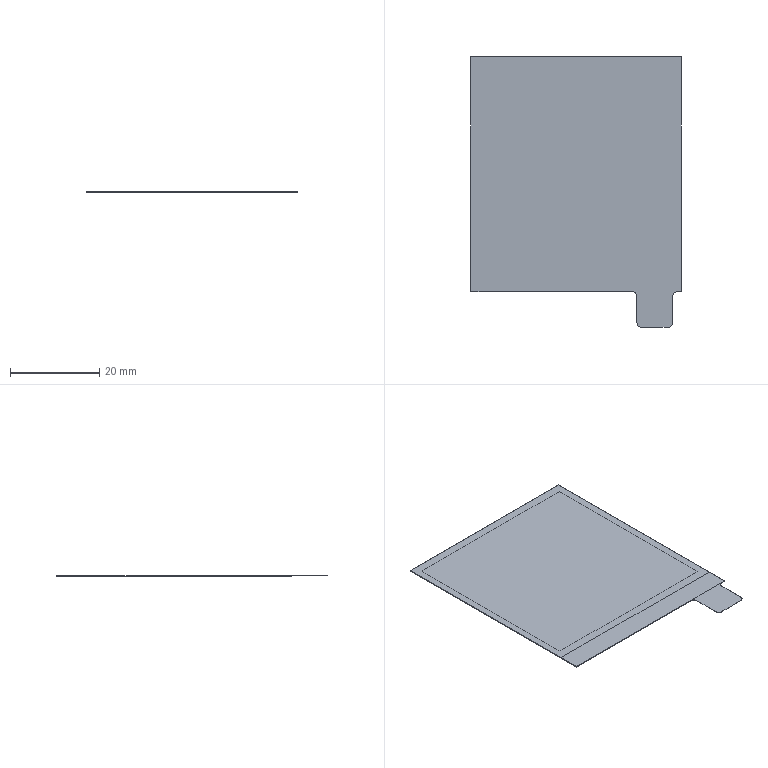Part | NX | features DATUM_CSYS 6, EXTRUDE 6, SKETCH 5 | 4 solids | 40 faces | box 47.2 x 60.8 x 0.18 mm | volume 184.569 mm3 | plane 36 | cylinder 4 | commonest cylinder face diameters 2 x4
STEP:
#1=CARTESIAN_POINT('',(0.,52.8,0.));
#2=VERTEX_POINT('',#1);
#3=CARTESIAN_POINT('',(0.,0.,0.));
#4=VERTEX_POINT('',#3);
#5=CARTESIAN_POINT('',(0.,52.8,0.));
#6=DIRECTION('',(0.,-1.,0.));
#7=VECTOR('',#6,1000.);
#8=LINE('',#5,#7);
#9=EDGE_CURVE('',#2,#4,#8,.T.);
#10=ORIENTED_EDGE('',*,*,#9,.F.);
#11=CARTESIAN_POINT('',(0.,52.8,-0.04));
#12=VERTEX_POINT('',#11);
#13=CARTESIAN_POINT('',(0.,52.8,-0.04));
#14=DIRECTION('',(0.,0.,1.));
#15=VECTOR('',#14,1000.);
#16=LINE('',#13,#15);
#17=EDGE_CURVE('',#12,#2,#16,.T.);
#18=ORIENTED_EDGE('',*,*,#17,.F.);
#19=CARTESIAN_POINT('',(0.,0.,-0.04));
#20=VERTEX_POINT('',#19);
#21=CARTESIAN_POINT('',(0.,52.8,-0.04));
#22=DIRECTION('',(0.,-1.,0.));
#23=VECTOR('',#22,1000.);
#24=LINE('',#21,#23);
#25=EDGE_CURVE('',#12,#20,#24,.T.);
#26=ORIENTED_EDGE('',*,*,#25,.T.);
#27=CARTESIAN_POINT('',(0.,0.,-0.04));
#28=DIRECTION('',(0.,0.,1.));
#29=VECTOR('',#28,1000.);
#30=LINE('',#27,#29);
#31=EDGE_CURVE('',#20,#4,#30,.T.);
#32=ORIENTED_EDGE('',*,*,#31,.T.);
#33=EDGE_LOOP('',(#10,#18,#26,#32));
#34=FACE_BOUND('',#33,.T.);
#35=CARTESIAN_POINT('',(0.,52.8,-0.04));
#36=DIRECTION('',(-1.,0.,0.));
#37=DIRECTION('',(0.,-1.,0.));
#38=AXIS2_PLACEMENT_3D('',#35,#36,#37);
#39=PLANE('',#38);
#40=ADVANCED_FACE('',(#34),#39,.T.);
#41=CARTESIAN_POINT('',(47.2,0.,0.));
#42=VERTEX_POINT('',#41);
#43=CARTESIAN_POINT('',(0.,0.,0.));
#44=DIRECTION('',(1.,0.,0.));
#45=VECTOR('',#44,1000.);
#46=LINE('',#43,#45);
#47=EDGE_CURVE('',#4,#42,#46,.T.);
#48=ORIENTED_EDGE('',*,*,#47,.F.);
#49=ORIENTED_EDGE('',*,*,#31,.F.);
#50=CARTESIAN_POINT('',(47.2,0.,-0.04));
#51=VERTEX_POINT('',#50);
#52=CARTESIAN_POINT('',(0.,0.,-0.04));
#53=DIRECTION('',(1.,0.,0.));
#54=VECTOR('',#53,1000.);
#55=LINE('',#52,#54);
#56=EDGE_CURVE('',#20,#51,#55,.T.);
#57=ORIENTED_EDGE('',*,*,#56,.T.);
#58=CARTESIAN_POINT('',(47.2,0.,-0.04));
#59=DIRECTION('',(0.,0.,1.));
#60=VECTOR('',#59,1000.);
#61=LINE('',#58,#60);
#62=EDGE_CURVE('',#51,#42,#61,.T.);
#63=ORIENTED_EDGE('',*,*,#62,.T.);
#64=EDGE_LOOP('',(#48,#49,#57,#63));
#65=FACE_BOUND('',#64,.T.);
#66=CARTESIAN_POINT('',(0.,0.,-0.04));
#67=DIRECTION('',(0.,-1.,0.));
#68=DIRECTION('',(0.,0.,-1.));
#69=AXIS2_PLACEMENT_3D('',#66,#67,#68);
#70=PLANE('',#69);
#71=ADVANCED_FACE('',(#65),#70,.T.);
#72=CARTESIAN_POINT('',(47.2,52.8,0.));
#73=VERTEX_POINT('',#72);
#74=CARTESIAN_POINT('',(47.2,0.,0.));
#75=DIRECTION('',(0.,1.,0.));
#76=VECTOR('',#75,1000.);
#77=LINE('',#74,#76);
#78=EDGE_CURVE('',#42,#73,#77,.T.);
#79=ORIENTED_EDGE('',*,*,#78,.F.);
#80=ORIENTED_EDGE('',*,*,#62,.F.);
#81=CARTESIAN_POINT('',(47.2,52.8,-0.04));
#82=VERTEX_POINT('',#81);
#83=CARTESIAN_POINT('',(47.2,0.,-0.04));
#84=DIRECTION('',(0.,1.,0.));
#85=VECTOR('',#84,1000.);
#86=LINE('',#83,#85);
#87=EDGE_CURVE('',#51,#82,#86,.T.);
#88=ORIENTED_EDGE('',*,*,#87,.T.);
#89=CARTESIAN_POINT('',(47.2,52.8,-0.04));
#90=DIRECTION('',(0.,0.,1.));
#91=VECTOR('',#90,1000.);
#92=LINE('',#89,#91);
#93=EDGE_CURVE('',#82,#73,#92,.T.);
#94=ORIENTED_EDGE('',*,*,#93,.T.);
#95=EDGE_LOOP('',(#79,#80,#88,#94));
#96=FACE_BOUND('',#95,.T.);
#97=CARTESIAN_POINT('',(47.2,0.,-0.04));
#98=DIRECTION('',(1.,0.,0.));
#99=DIRECTION('',(0.,0.,-1.));
#100=AXIS2_PLACEMENT_3D('',#97,#98,#99);
#101=PLANE('',#100);
#102=ADVANCED_FACE('',(#96),#101,.T.);
#103=CARTESIAN_POINT('',(47.2,52.8,0.));
#104=DIRECTION('',(-1.,0.,0.));
#105=VECTOR('',#104,1000.);
#106=LINE('',#103,#105);
#107=EDGE_CURVE('',#73,#2,#106,.T.);
#108=ORIENTED_EDGE('',*,*,#107,.F.);
#109=ORIENTED_EDGE('',*,*,#93,.F.);
#110=CARTESIAN_POINT('',(47.2,52.8,-0.04));
#111=DIRECTION('',(-1.,0.,0.));
#112=VECTOR('',#111,1000.);
#113=LINE('',#110,#112);
#114=EDGE_CURVE('',#82,#12,#113,.T.);
#115=ORIENTED_EDGE('',*,*,#114,.T.);
#116=ORIENTED_EDGE('',*,*,#17,.T.);
#117=EDGE_LOOP('',(#108,#109,#115,#116));
#118=FACE_BOUND('',#117,.T.);
#119=CARTESIAN_POINT('',(47.2,52.8,-0.04));
#120=DIRECTION('',(0.,1.,0.));
#121=DIRECTION('',(-1.,0.,0.));
#122=AXIS2_PLACEMENT_3D('',#119,#120,#121);
#123=PLANE('',#122);
#124=ADVANCED_FACE('',(#118),#123,.T.);
#125=CARTESIAN_POINT('',(45.5,50.9,-0.04));
#126=VERTEX_POINT('',#125);
#127=CARTESIAN_POINT('',(1.7,50.9,-0.04));
#128=VERTEX_POINT('',#127);
#129=CARTESIAN_POINT('',(0.,50.9,-0.04));
#130=DIRECTION('',(-1.,0.,0.));
#131=VECTOR('',#130,1000.);
#132=LINE('',#129,#131);
#133=EDGE_CURVE('',#126,#128,#132,.T.);
#134=ORIENTED_EDGE('',*,*,#133,.T.);
#135=CARTESIAN_POINT('',(1.7,6.9,-0.04));
#136=VERTEX_POINT('',#135);
#137=CARTESIAN_POINT('',(1.7,0.,-0.04));
#138=DIRECTION('',(0.,-1.,0.));
#139=VECTOR('',#138,1000.);
#140=LINE('',#137,#139);
#141=EDGE_CURVE('',#128,#136,#140,.T.);
#142=ORIENTED_EDGE('',*,*,#141,.T.);
#143=CARTESIAN_POINT('',(45.5,6.9,-0.04));
#144=VERTEX_POINT('',#143);
#145=CARTESIAN_POINT('',(0.,6.9,-0.04));
#146=DIRECTION('',(1.,0.,0.));
#147=VECTOR('',#146,1000.);
#148=LINE('',#145,#147);
#149=EDGE_CURVE('',#136,#144,#148,.T.);
#150=ORIENTED_EDGE('',*,*,#149,.T.);
#151=CARTESIAN_POINT('',(45.5,0.,-0.04));
#152=DIRECTION('',(0.,1.,0.));
#153=VECTOR('',#152,1000.);
#154=LINE('',#151,#153);
#155=EDGE_CURVE('',#144,#126,#154,.T.);
#156=ORIENTED_EDGE('',*,*,#155,.T.);
#157=EDGE_LOOP('',(#134,#142,#150,#156));
#158=FACE_BOUND('',#157,.T.);
#159=ORIENTED_EDGE('',*,*,#25,.F.);
#160=ORIENTED_EDGE('',*,*,#114,.F.);
#161=ORIENTED_EDGE('',*,*,#87,.F.);
#162=ORIENTED_EDGE('',*,*,#56,.F.);
#163=EDGE_LOOP('',(#159,#160,#161,#162));
#164=FACE_BOUND('',#163,.T.);
#165=CARTESIAN_POINT('',(0.,0.,-0.04));
#166=DIRECTION('',(0.,0.,1.));
#167=DIRECTION('',(1.,0.,0.));
#168=AXIS2_PLACEMENT_3D('',#165,#166,#167);
#169=PLANE('',#168);
#170=ADVANCED_FACE('',(#158,#164),#169,.F.);
#171=CARTESIAN_POINT('',(1.7,50.9,0.));
#172=VERTEX_POINT('',#171);
#173=CARTESIAN_POINT('',(1.7,6.9,0.));
#174=VERTEX_POINT('',#173);
#175=CARTESIAN_POINT('',(1.7,0.,0.));
#176=DIRECTION('',(0.,-1.,0.));
#177=VECTOR('',#176,1000.);
#178=LINE('',#175,#177);
#179=EDGE_CURVE('',#172,#174,#178,.T.);
#180=ORIENTED_EDGE('',*,*,#179,.F.);
#181=CARTESIAN_POINT('',(45.5,50.9,0.));
#182=VERTEX_POINT('',#181);
#183=CARTESIAN_POINT('',(0.,50.9,0.));
#184=DIRECTION('',(-1.,0.,0.));
#185=VECTOR('',#184,1000.);
#186=LINE('',#183,#185);
#187=EDGE_CURVE('',#182,#172,#186,.T.);
#188=ORIENTED_EDGE('',*,*,#187,.F.);
#189=CARTESIAN_POINT('',(45.5,6.9,0.));
#190=VERTEX_POINT('',#189);
#191=CARTESIAN_POINT('',(45.5,0.,0.));
#192=DIRECTION('',(0.,1.,0.));
#193=VECTOR('',#192,1000.);
#194=LINE('',#191,#193);
#195=EDGE_CURVE('',#190,#182,#194,.T.);
#196=ORIENTED_EDGE('',*,*,#195,.F.);
#197=CARTESIAN_POINT('',(0.,6.9,0.));
#198=DIRECTION('',(1.,0.,0.));
#199=VECTOR('',#198,1000.);
#200=LINE('',#197,#199);
#201=EDGE_CURVE('',#174,#190,#200,.T.);
#202=ORIENTED_EDGE('',*,*,#201,.F.);
#203=EDGE_LOOP('',(#180,#188,#196,#202));
#204=FACE_BOUND('',#203,.T.);
#205=ORIENTED_EDGE('',*,*,#9,.T.);
#206=ORIENTED_EDGE('',*,*,#47,.T.);
#207=ORIENTED_EDGE('',*,*,#78,.T.);
#208=ORIENTED_EDGE('',*,*,#107,.T.);
#209=EDGE_LOOP('',(#205,#206,#207,#208));
#210=FACE_BOUND('',#209,.T.);
#211=CARTESIAN_POINT('',(0.,0.,0.));
#212=DIRECTION('',(0.,0.,1.));
#213=DIRECTION('',(1.,0.,0.));
#214=AXIS2_PLACEMENT_3D('',#211,#212,#213);
#215=PLANE('',#214);
#216=ADVANCED_FACE('',(#204,#210),#215,.T.);
#217=CARTESIAN_POINT('',(1.7,50.9,1.05));
#218=DIRECTION('',(0.,0.,-1.));
#219=VECTOR('',#218,1000.);
#220=LINE('',#217,#219);
#221=EDGE_CURVE('',#128,#172,#220,.F.);
#222=ORIENTED_EDGE('',*,*,#221,.T.);
#223=ORIENTED_EDGE('',*,*,#179,.T.);
#224=CARTESIAN_POINT('',(1.7,6.9,1.05));
#225=DIRECTION('',(0.,0.,-1.));
#226=VECTOR('',#225,1000.);
#227=LINE('',#224,#226);
#228=EDGE_CURVE('',#136,#174,#227,.F.);
#229=ORIENTED_EDGE('',*,*,#228,.F.);
#230=ORIENTED_EDGE('',*,*,#141,.F.);
#231=EDGE_LOOP('',(#222,#223,#229,#230));
#232=FACE_BOUND('',#231,.T.);
#233=CARTESIAN_POINT('',(1.7,6.9,1.05));
#234=DIRECTION('',(-1.,0.,0.));
#235=DIRECTION('',(0.,-1.,0.));
#236=AXIS2_PLACEMENT_3D('',#233,#234,#235);
#237=PLANE('',#236);
#238=ADVANCED_FACE('',(#232),#237,.F.);
#239=CARTESIAN_POINT('',(45.5,50.9,1.05));
#240=DIRECTION('',(0.,0.,-1.));
#241=VECTOR('',#240,1000.);
#242=LINE('',#239,#241);
#243=EDGE_CURVE('',#126,#182,#242,.F.);
#244=ORIENTED_EDGE('',*,*,#243,.T.);
#245=ORIENTED_EDGE('',*,*,#187,.T.);
#246=ORIENTED_EDGE('',*,*,#221,.F.);
#247=ORIENTED_EDGE('',*,*,#133,.F.);
#248=EDGE_LOOP('',(#244,#245,#246,#247));
#249=FACE_BOUND('',#248,.T.);
#250=CARTESIAN_POINT('',(1.7,50.9,1.05));
#251=DIRECTION('',(0.,1.,0.));
#252=DIRECTION('',(-1.,0.,0.));
#253=AXIS2_PLACEMENT_3D('',#250,#251,#252);
#254=PLANE('',#253);
#255=ADVANCED_FACE('',(#249),#254,.F.);
#256=CARTESIAN_POINT('',(45.5,6.9,1.05));
#257=DIRECTION('',(0.,0.,-1.));
#258=VECTOR('',#257,1000.);
#259=LINE('',#256,#258);
#260=EDGE_CURVE('',#144,#190,#259,.F.);
#261=ORIENTED_EDGE('',*,*,#260,.T.);
#262=ORIENTED_EDGE('',*,*,#195,.T.);
#263=ORIENTED_EDGE('',*,*,#243,.F.);
#264=ORIENTED_EDGE('',*,*,#155,.F.);
#265=EDGE_LOOP('',(#261,#262,#263,#264));
#266=FACE_BOUND('',#265,.T.);
#267=CARTESIAN_POINT('',(45.5,50.9,1.05));
#268=DIRECTION('',(1.,0.,0.));
#269=DIRECTION('',(0.,1.,0.));
#270=AXIS2_PLACEMENT_3D('',#267,#268,#269);
#271=PLANE('',#270);
#272=ADVANCED_FACE('',(#266),#271,.F.);
#273=ORIENTED_EDGE('',*,*,#228,.T.);
#274=ORIENTED_EDGE('',*,*,#201,.T.);
#275=ORIENTED_EDGE('',*,*,#260,.F.);
#276=ORIENTED_EDGE('',*,*,#149,.F.);
#277=EDGE_LOOP('',(#273,#274,#275,#276));
#278=FACE_BOUND('',#277,.T.);
#279=CARTESIAN_POINT('',(45.5,6.9,1.05));
#280=DIRECTION('',(0.,-1.,0.));
#281=DIRECTION('',(1.,0.,0.));
#282=AXIS2_PLACEMENT_3D('',#279,#280,#281);
#283=PLANE('',#282);
#284=ADVANCED_FACE('',(#278),#283,.F.);
#285=CLOSED_SHELL('',(#40,#71,#102,#124,#170,#216,#238,#255,#272,#284));
#286=MANIFOLD_SOLID_BREP('',#285);
#287=CARTESIAN_POINT('',(0.,0.,-0.08));
#288=VERTEX_POINT('',#287);
#289=CARTESIAN_POINT('',(0.,52.8,-0.08));
#290=VERTEX_POINT('',#289);
#291=CARTESIAN_POINT('',(0.,0.,-0.08));
#292=DIRECTION('',(0.,1.,0.));
#293=VECTOR('',#292,1000.);
#294=LINE('',#291,#293);
#295=EDGE_CURVE('',#288,#290,#294,.T.);
#296=ORIENTED_EDGE('',*,*,#295,.T.);
#297=CARTESIAN_POINT('',(47.2,52.8,-0.08));
#298=VERTEX_POINT('',#297);
#299=CARTESIAN_POINT('',(0.,52.8,-0.08));
#300=DIRECTION('',(1.,0.,0.));
#301=VECTOR('',#300,1000.);
#302=LINE('',#299,#301);
#303=EDGE_CURVE('',#290,#298,#302,.T.);
#304=ORIENTED_EDGE('',*,*,#303,.T.);
#305=CARTESIAN_POINT('',(47.2,0.,-0.08));
#306=VERTEX_POINT('',#305);
#307=CARTESIAN_POINT('',(47.2,52.8,-0.08));
#308=DIRECTION('',(0.,-1.,0.));
#309=VECTOR('',#308,1000.);
#310=LINE('',#307,#309);
#311=EDGE_CURVE('',#298,#306,#310,.T.);
#312=ORIENTED_EDGE('',*,*,#311,.T.);
#313=CARTESIAN_POINT('',(47.2,0.,-0.08));
#314=DIRECTION('',(-1.,0.,0.));
#315=VECTOR('',#314,1000.);
#316=LINE('',#313,#315);
#317=EDGE_CURVE('',#306,#288,#316,.T.);
#318=ORIENTED_EDGE('',*,*,#317,.T.);
#319=EDGE_LOOP('',(#296,#304,#312,#318));
#320=FACE_BOUND('',#319,.T.);
#321=CARTESIAN_POINT('',(45.5,50.9,-0.08));
#322=VERTEX_POINT('',#321);
#323=CARTESIAN_POINT('',(1.7,50.9,-0.08));
#324=VERTEX_POINT('',#323);
#325=CARTESIAN_POINT('',(0.,50.9,-0.08));
#326=DIRECTION('',(-1.,0.,0.));
#327=VECTOR('',#326,1000.);
#328=LINE('',#325,#327);
#329=EDGE_CURVE('',#322,#324,#328,.T.);
#330=ORIENTED_EDGE('',*,*,#329,.T.);
#331=CARTESIAN_POINT('',(1.7,6.9,-0.08));
#332=VERTEX_POINT('',#331);
#333=CARTESIAN_POINT('',(1.7,0.,-0.08));
#334=DIRECTION('',(0.,-1.,0.));
#335=VECTOR('',#334,1000.);
#336=LINE('',#333,#335);
#337=EDGE_CURVE('',#324,#332,#336,.T.);
#338=ORIENTED_EDGE('',*,*,#337,.T.);
#339=CARTESIAN_POINT('',(45.5,6.9,-0.08));
#340=VERTEX_POINT('',#339);
#341=CARTESIAN_POINT('',(0.,6.9,-0.08));
#342=DIRECTION('',(1.,0.,0.));
#343=VECTOR('',#342,1000.);
#344=LINE('',#341,#343);
#345=EDGE_CURVE('',#332,#340,#344,.T.);
#346=ORIENTED_EDGE('',*,*,#345,.T.);
#347=CARTESIAN_POINT('',(45.5,0.,-0.08));
#348=DIRECTION('',(0.,1.,0.));
#349=VECTOR('',#348,1000.);
#350=LINE('',#347,#349);
#351=EDGE_CURVE('',#340,#322,#350,.T.);
#352=ORIENTED_EDGE('',*,*,#351,.T.);
#353=EDGE_LOOP('',(#330,#338,#346,#352));
#354=FACE_BOUND('',#353,.T.);
#355=CARTESIAN_POINT('',(0.,0.,-0.08));
#356=DIRECTION('',(0.,0.,-1.));
#357=DIRECTION('',(-1.,0.,0.));
#358=AXIS2_PLACEMENT_3D('',#355,#356,#357);
#359=PLANE('',#358);
#360=ADVANCED_FACE('',(#320,#354),#359,.T.);
#361=CARTESIAN_POINT('',(0.,0.,-0.04));
#362=VERTEX_POINT('',#361);
#363=CARTESIAN_POINT('',(0.,52.8,-0.04));
#364=VERTEX_POINT('',#363);
#365=CARTESIAN_POINT('',(0.,0.,-0.04));
#366=DIRECTION('',(0.,1.,0.));
#367=VECTOR('',#366,1000.);
#368=LINE('',#365,#367);
#369=EDGE_CURVE('',#362,#364,#368,.T.);
#370=ORIENTED_EDGE('',*,*,#369,.F.);
#371=CARTESIAN_POINT('',(47.2,0.,-0.04));
#372=VERTEX_POINT('',#371);
#373=CARTESIAN_POINT('',(47.2,0.,-0.04));
#374=DIRECTION('',(-1.,0.,0.));
#375=VECTOR('',#374,1000.);
#376=LINE('',#373,#375);
#377=EDGE_CURVE('',#372,#362,#376,.T.);
#378=ORIENTED_EDGE('',*,*,#377,.F.);
#379=CARTESIAN_POINT('',(47.2,52.8,-0.04));
#380=VERTEX_POINT('',#379);
#381=CARTESIAN_POINT('',(47.2,52.8,-0.04));
#382=DIRECTION('',(0.,-1.,0.));
#383=VECTOR('',#382,1000.);
#384=LINE('',#381,#383);
#385=EDGE_CURVE('',#380,#372,#384,.T.);
#386=ORIENTED_EDGE('',*,*,#385,.F.);
#387=CARTESIAN_POINT('',(0.,52.8,-0.04));
#388=DIRECTION('',(1.,0.,0.));
#389=VECTOR('',#388,1000.);
#390=LINE('',#387,#389);
#391=EDGE_CURVE('',#364,#380,#390,.T.);
#392=ORIENTED_EDGE('',*,*,#391,.F.);
#393=EDGE_LOOP('',(#370,#378,#386,#392));
#394=FACE_BOUND('',#393,.T.);
#395=CARTESIAN_POINT('',(1.7,50.9,-0.04));
#396=VERTEX_POINT('',#395);
#397=CARTESIAN_POINT('',(1.7,6.9,-0.04));
#398=VERTEX_POINT('',#397);
#399=CARTESIAN_POINT('',(1.7,0.,-0.04));
#400=DIRECTION('',(0.,-1.,0.));
#401=VECTOR('',#400,1000.);
#402=LINE('',#399,#401);
#403=EDGE_CURVE('',#396,#398,#402,.T.);
#404=ORIENTED_EDGE('',*,*,#403,.F.);
#405=CARTESIAN_POINT('',(45.5,50.9,-0.04));
#406=VERTEX_POINT('',#405);
#407=CARTESIAN_POINT('',(0.,50.9,-0.04));
#408=DIRECTION('',(-1.,0.,0.));
#409=VECTOR('',#408,1000.);
#410=LINE('',#407,#409);
#411=EDGE_CURVE('',#406,#396,#410,.T.);
#412=ORIENTED_EDGE('',*,*,#411,.F.);
#413=CARTESIAN_POINT('',(45.5,6.9,-0.04));
#414=VERTEX_POINT('',#413);
#415=CARTESIAN_POINT('',(45.5,0.,-0.04));
#416=DIRECTION('',(0.,1.,0.));
#417=VECTOR('',#416,1000.);
#418=LINE('',#415,#417);
#419=EDGE_CURVE('',#414,#406,#418,.T.);
#420=ORIENTED_EDGE('',*,*,#419,.F.);
#421=CARTESIAN_POINT('',(0.,6.9,-0.04));
#422=DIRECTION('',(1.,0.,0.));
#423=VECTOR('',#422,1000.);
#424=LINE('',#421,#423);
#425=EDGE_CURVE('',#398,#414,#424,.T.);
#426=ORIENTED_EDGE('',*,*,#425,.F.);
#427=EDGE_LOOP('',(#404,#412,#420,#426));
#428=FACE_BOUND('',#427,.T.);
#429=CARTESIAN_POINT('',(0.,0.,-0.04));
#430=DIRECTION('',(0.,0.,-1.));
#431=DIRECTION('',(-1.,0.,0.));
#432=AXIS2_PLACEMENT_3D('',#429,#430,#431);
#433=PLANE('',#432);
#434=ADVANCED_FACE('',(#394,#428),#433,.F.);
#435=ORIENTED_EDGE('',*,*,#369,.T.);
#436=CARTESIAN_POINT('',(0.,52.8,-0.08));
#437=DIRECTION('',(0.,0.,1.));
#438=VECTOR('',#437,1000.);
#439=LINE('',#436,#438);
#440=EDGE_CURVE('',#290,#364,#439,.T.);
#441=ORIENTED_EDGE('',*,*,#440,.F.);
#442=ORIENTED_EDGE('',*,*,#295,.F.);
#443=CARTESIAN_POINT('',(0.,0.,-0.08));
#444=DIRECTION('',(0.,0.,1.));
#445=VECTOR('',#444,1000.);
#446=LINE('',#443,#445);
#447=EDGE_CURVE('',#288,#362,#446,.T.);
#448=ORIENTED_EDGE('',*,*,#447,.T.);
#449=EDGE_LOOP('',(#435,#441,#442,#448));
#450=FACE_BOUND('',#449,.T.);
#451=CARTESIAN_POINT('',(0.,0.,-0.08));
#452=DIRECTION('',(1.,0.,0.));
#453=DIRECTION('',(0.,0.,-1.));
#454=AXIS2_PLACEMENT_3D('',#451,#452,#453);
#455=PLANE('',#454);
#456=ADVANCED_FACE('',(#450),#455,.F.);
#457=ORIENTED_EDGE('',*,*,#391,.T.);
#458=CARTESIAN_POINT('',(47.2,52.8,-0.08));
#459=DIRECTION('',(0.,0.,1.));
#460=VECTOR('',#459,1000.);
#461=LINE('',#458,#460);
#462=EDGE_CURVE('',#298,#380,#461,.T.);
#463=ORIENTED_EDGE('',*,*,#462,.F.);
#464=ORIENTED_EDGE('',*,*,#303,.F.);
#465=ORIENTED_EDGE('',*,*,#440,.T.);
#466=EDGE_LOOP('',(#457,#463,#464,#465));
#467=FACE_BOUND('',#466,.T.);
#468=CARTESIAN_POINT('',(0.,52.8,-0.08));
#469=DIRECTION('',(0.,-1.,0.));
#470=DIRECTION('',(0.,0.,-1.));
#471=AXIS2_PLACEMENT_3D('',#468,#469,#470);
#472=PLANE('',#471);
#473=ADVANCED_FACE('',(#467),#472,.F.);
#474=ORIENTED_EDGE('',*,*,#385,.T.);
#475=CARTESIAN_POINT('',(47.2,0.,-0.08));
#476=DIRECTION('',(0.,0.,1.));
#477=VECTOR('',#476,1000.);
#478=LINE('',#475,#477);
#479=EDGE_CURVE('',#306,#372,#478,.T.);
#480=ORIENTED_EDGE('',*,*,#479,.F.);
#481=ORIENTED_EDGE('',*,*,#311,.F.);
#482=ORIENTED_EDGE('',*,*,#462,.T.);
#483=EDGE_LOOP('',(#474,#480,#481,#482));
#484=FACE_BOUND('',#483,.T.);
#485=CARTESIAN_POINT('',(47.2,52.8,-0.08));
#486=DIRECTION('',(-1.,0.,0.));
#487=DIRECTION('',(0.,0.,1.));
#488=AXIS2_PLACEMENT_3D('',#485,#486,#487);
#489=PLANE('',#488);
#490=ADVANCED_FACE('',(#484),#489,.F.);
#491=ORIENTED_EDGE('',*,*,#377,.T.);
#492=ORIENTED_EDGE('',*,*,#447,.F.);
#493=ORIENTED_EDGE('',*,*,#317,.F.);
#494=ORIENTED_EDGE('',*,*,#479,.T.);
#495=EDGE_LOOP('',(#491,#492,#493,#494));
#496=FACE_BOUND('',#495,.T.);
#497=CARTESIAN_POINT('',(47.2,0.,-0.08));
#498=DIRECTION('',(0.,1.,0.));
#499=DIRECTION('',(0.,0.,1.));
#500=AXIS2_PLACEMENT_3D('',#497,#498,#499);
#501=PLANE('',#500);
#502=ADVANCED_FACE('',(#496),#501,.F.);
#503=CARTESIAN_POINT('',(1.7,50.9,1.05));
#504=DIRECTION('',(0.,0.,-1.));
#505=VECTOR('',#504,1000.);
#506=LINE('',#503,#505);
#507=EDGE_CURVE('',#324,#396,#506,.F.);
#508=ORIENTED_EDGE('',*,*,#507,.T.);
#509=ORIENTED_EDGE('',*,*,#403,.T.);
#510=CARTESIAN_POINT('',(1.7,6.9,1.05));
#511=DIRECTION('',(0.,0.,-1.));
#512=VECTOR('',#511,1000.);
#513=LINE('',#510,#512);
#514=EDGE_CURVE('',#332,#398,#513,.F.);
#515=ORIENTED_EDGE('',*,*,#514,.F.);
#516=ORIENTED_EDGE('',*,*,#337,.F.);
#517=EDGE_LOOP('',(#508,#509,#515,#516));
#518=FACE_BOUND('',#517,.T.);
#519=CARTESIAN_POINT('',(1.7,50.9,1.05));
#520=DIRECTION('',(1.,0.,0.));
#521=DIRECTION('',(0.,1.,0.));
#522=AXIS2_PLACEMENT_3D('',#519,#520,#521);
#523=PLANE('',#522);
#524=ADVANCED_FACE('',(#518),#523,.T.);
#525=ORIENTED_EDGE('',*,*,#514,.T.);
#526=ORIENTED_EDGE('',*,*,#425,.T.);
#527=CARTESIAN_POINT('',(45.5,6.9,1.05));
#528=DIRECTION('',(0.,0.,-1.));
#529=VECTOR('',#528,1000.);
#530=LINE('',#527,#529);
#531=EDGE_CURVE('',#340,#414,#530,.F.);
#532=ORIENTED_EDGE('',*,*,#531,.F.);
#533=ORIENTED_EDGE('',*,*,#345,.F.);
#534=EDGE_LOOP('',(#525,#526,#532,#533));
#535=FACE_BOUND('',#534,.T.);
#536=CARTESIAN_POINT('',(1.7,6.9,1.05));
#537=DIRECTION('',(0.,1.,0.));
#538=DIRECTION('',(-1.,0.,0.));
#539=AXIS2_PLACEMENT_3D('',#536,#537,#538);
#540=PLANE('',#539);
#541=ADVANCED_FACE('',(#535),#540,.T.);
#542=ORIENTED_EDGE('',*,*,#531,.T.);
#543=ORIENTED_EDGE('',*,*,#419,.T.);
#544=CARTESIAN_POINT('',(45.5,50.9,1.05));
#545=DIRECTION('',(0.,0.,-1.));
#546=VECTOR('',#545,1000.);
#547=LINE('',#544,#546);
#548=EDGE_CURVE('',#322,#406,#547,.F.);
#549=ORIENTED_EDGE('',*,*,#548,.F.);
#550=ORIENTED_EDGE('',*,*,#351,.F.);
#551=EDGE_LOOP('',(#542,#543,#549,#550));
#552=FACE_BOUND('',#551,.T.);
#553=CARTESIAN_POINT('',(45.5,6.9,1.05));
#554=DIRECTION('',(-1.,0.,0.));
#555=DIRECTION('',(0.,-1.,0.));
#556=AXIS2_PLACEMENT_3D('',#553,#554,#555);
#557=PLANE('',#556);
#558=ADVANCED_FACE('',(#552),#557,.T.);
#559=ORIENTED_EDGE('',*,*,#548,.T.);
#560=ORIENTED_EDGE('',*,*,#411,.T.);
#561=ORIENTED_EDGE('',*,*,#507,.F.);
#562=ORIENTED_EDGE('',*,*,#329,.F.);
#563=EDGE_LOOP('',(#559,#560,#561,#562));
#564=FACE_BOUND('',#563,.T.);
#565=CARTESIAN_POINT('',(45.5,50.9,1.05));
#566=DIRECTION('',(0.,-1.,0.));
#567=DIRECTION('',(1.,0.,0.));
#568=AXIS2_PLACEMENT_3D('',#565,#566,#567);
#569=PLANE('',#568);
#570=ADVANCED_FACE('',(#564),#569,.T.);
#571=CLOSED_SHELL('',(#360,#434,#456,#473,#490,#502,#524,#541,#558,#570));
#572=MANIFOLD_SOLID_BREP('',#571);
#573=CARTESIAN_POINT('',(0.,52.8,0.05));
#574=VERTEX_POINT('',#573);
#575=CARTESIAN_POINT('',(0.,0.,0.05));
#576=VERTEX_POINT('',#575);
#577=CARTESIAN_POINT('',(0.,52.8,0.05));
#578=DIRECTION('',(0.,-1.,0.));
#579=VECTOR('',#578,1000.);
#580=LINE('',#577,#579);
#581=EDGE_CURVE('',#574,#576,#580,.T.);
#582=ORIENTED_EDGE('',*,*,#581,.T.);
#583=CARTESIAN_POINT('',(0.,0.,0.1));
#584=VERTEX_POINT('',#583);
#585=CARTESIAN_POINT('',(0.,0.,0.1));
#586=DIRECTION('',(0.,0.,-1.));
#587=VECTOR('',#586,1000.);
#588=LINE('',#585,#587);
#589=EDGE_CURVE('',#584,#576,#588,.T.);
#590=ORIENTED_EDGE('',*,*,#589,.F.);
#591=CARTESIAN_POINT('',(0.,52.8,0.1));
#592=VERTEX_POINT('',#591);
#593=CARTESIAN_POINT('',(0.,52.8,0.1));
#594=DIRECTION('',(0.,-1.,0.));
#595=VECTOR('',#594,1000.);
#596=LINE('',#593,#595);
#597=EDGE_CURVE('',#592,#584,#596,.T.);
#598=ORIENTED_EDGE('',*,*,#597,.F.);
#599=CARTESIAN_POINT('',(0.,52.8,0.1));
#600=DIRECTION('',(0.,0.,-1.));
#601=VECTOR('',#600,1000.);
#602=LINE('',#599,#601);
#603=EDGE_CURVE('',#592,#574,#602,.T.);
#604=ORIENTED_EDGE('',*,*,#603,.T.);
#605=EDGE_LOOP('',(#582,#590,#598,#604));
#606=FACE_BOUND('',#605,.T.);
#607=CARTESIAN_POINT('',(0.,52.8,0.1));
#608=DIRECTION('',(1.,0.,0.));
#609=DIRECTION('',(0.,0.,-1.));
#610=AXIS2_PLACEMENT_3D('',#607,#608,#609);
#611=PLANE('',#610);
#612=ADVANCED_FACE('',(#606),#611,.F.);
#613=CARTESIAN_POINT('',(36.3,0.,0.05));
#614=VERTEX_POINT('',#613);
#615=CARTESIAN_POINT('',(0.,0.,0.05));
#616=DIRECTION('',(1.,0.,0.));
#617=VECTOR('',#616,1000.);
#618=LINE('',#615,#617);
#619=EDGE_CURVE('',#576,#614,#618,.T.);
#620=ORIENTED_EDGE('',*,*,#619,.T.);
#621=CARTESIAN_POINT('',(36.3,0.,0.1));
#622=VERTEX_POINT('',#621);
#623=CARTESIAN_POINT('',(36.3,0.,0.1));
#624=DIRECTION('',(0.,0.,-1.));
#625=VECTOR('',#624,1000.);
#626=LINE('',#623,#625);
#627=EDGE_CURVE('',#622,#614,#626,.T.);
#628=ORIENTED_EDGE('',*,*,#627,.F.);
#629=CARTESIAN_POINT('',(0.,0.,0.1));
#630=DIRECTION('',(1.,0.,0.));
#631=VECTOR('',#630,1000.);
#632=LINE('',#629,#631);
#633=EDGE_CURVE('',#584,#622,#632,.T.);
#634=ORIENTED_EDGE('',*,*,#633,.F.);
#635=ORIENTED_EDGE('',*,*,#589,.T.);
#636=EDGE_LOOP('',(#620,#628,#634,#635));
#637=FACE_BOUND('',#636,.T.);
#638=CARTESIAN_POINT('',(0.,0.,0.1));
#639=DIRECTION('',(0.,1.,0.));
#640=DIRECTION('',(0.,0.,1.));
#641=AXIS2_PLACEMENT_3D('',#638,#639,#640);
#642=PLANE('',#641);
#643=ADVANCED_FACE('',(#637),#642,.F.);
#644=CARTESIAN_POINT('',(37.3,-1.,0.05));
#645=VERTEX_POINT('',#644);
#646=CARTESIAN_POINT('',(36.3,-1.,0.05));
#647=DIRECTION('',(0.,0.,-1.));
#648=DIRECTION('',(0.,1.,0.));
#649=AXIS2_PLACEMENT_3D('',#646,#647,#648);
#650=CIRCLE('',#649,1.);
#651=EDGE_CURVE('',#614,#645,#650,.T.);
#652=ORIENTED_EDGE('',*,*,#651,.T.);
#653=CARTESIAN_POINT('',(37.3,-1.,0.1));
#654=VERTEX_POINT('',#653);
#655=CARTESIAN_POINT('',(37.3,-1.,0.1));
#656=DIRECTION('',(0.,0.,-1.));
#657=VECTOR('',#656,1000.);
#658=LINE('',#655,#657);
#659=EDGE_CURVE('',#654,#645,#658,.T.);
#660=ORIENTED_EDGE('',*,*,#659,.F.);
#661=CARTESIAN_POINT('',(36.3,-1.,0.1));
#662=DIRECTION('',(0.,0.,-1.));
#663=DIRECTION('',(0.,1.,0.));
#664=AXIS2_PLACEMENT_3D('',#661,#662,#663);
#665=CIRCLE('',#664,1.);
#666=EDGE_CURVE('',#622,#654,#665,.T.);
#667=ORIENTED_EDGE('',*,*,#666,.F.);
#668=ORIENTED_EDGE('',*,*,#627,.T.);
#669=EDGE_LOOP('',(#652,#660,#667,#668));
#670=FACE_BOUND('',#669,.T.);
#671=CARTESIAN_POINT('',(36.3,-1.,0.1));
#672=DIRECTION('',(0.,0.,-1.));
#673=DIRECTION('',(-1.,0.,0.));
#674=AXIS2_PLACEMENT_3D('',#671,#672,#673);
#675=CYLINDRICAL_SURFACE('',#674,1.);
#676=ADVANCED_FACE('',(#670),#675,.F.);
#677=CARTESIAN_POINT('',(37.3,-7.,0.05));
#678=VERTEX_POINT('',#677);
#679=CARTESIAN_POINT('',(37.3,-1.,0.05));
#680=DIRECTION('',(0.,-1.,0.));
#681=VECTOR('',#680,1000.);
#682=LINE('',#679,#681);
#683=EDGE_CURVE('',#645,#678,#682,.T.);
#684=ORIENTED_EDGE('',*,*,#683,.T.);
#685=CARTESIAN_POINT('',(37.3,-7.,0.1));
#686=VERTEX_POINT('',#685);
#687=CARTESIAN_POINT('',(37.3,-7.,0.1));
#688=DIRECTION('',(0.,0.,-1.));
#689=VECTOR('',#688,1000.);
#690=LINE('',#687,#689);
#691=EDGE_CURVE('',#686,#678,#690,.T.);
#692=ORIENTED_EDGE('',*,*,#691,.F.);
#693=CARTESIAN_POINT('',(37.3,-1.,0.1));
#694=DIRECTION('',(0.,-1.,0.));
#695=VECTOR('',#694,1000.);
#696=LINE('',#693,#695);
#697=EDGE_CURVE('',#654,#686,#696,.T.);
#698=ORIENTED_EDGE('',*,*,#697,.F.);
#699=ORIENTED_EDGE('',*,*,#659,.T.);
#700=EDGE_LOOP('',(#684,#692,#698,#699));
#701=FACE_BOUND('',#700,.T.);
#702=CARTESIAN_POINT('',(37.3,-1.,0.1));
#703=DIRECTION('',(1.,0.,0.));
#704=DIRECTION('',(0.,1.,0.));
#705=AXIS2_PLACEMENT_3D('',#702,#703,#704);
#706=PLANE('',#705);
#707=ADVANCED_FACE('',(#701),#706,.F.);
#708=CARTESIAN_POINT('',(38.3,-8.,0.05));
#709=VERTEX_POINT('',#708);
#710=CARTESIAN_POINT('',(38.3,-7.,0.05));
#711=DIRECTION('',(0.,0.,1.));
#712=DIRECTION('',(0.,1.,0.));
#713=AXIS2_PLACEMENT_3D('',#710,#711,#712);
#714=CIRCLE('',#713,1.);
#715=EDGE_CURVE('',#678,#709,#714,.T.);
#716=ORIENTED_EDGE('',*,*,#715,.T.);
#717=CARTESIAN_POINT('',(38.3,-8.,0.1));
#718=VERTEX_POINT('',#717);
#719=CARTESIAN_POINT('',(38.3,-8.,0.1));
#720=DIRECTION('',(0.,0.,-1.));
#721=VECTOR('',#720,1000.);
#722=LINE('',#719,#721);
#723=EDGE_CURVE('',#718,#709,#722,.T.);
#724=ORIENTED_EDGE('',*,*,#723,.F.);
#725=CARTESIAN_POINT('',(38.3,-7.,0.1));
#726=DIRECTION('',(0.,0.,1.));
#727=DIRECTION('',(0.,1.,0.));
#728=AXIS2_PLACEMENT_3D('',#725,#726,#727);
#729=CIRCLE('',#728,1.);
#730=EDGE_CURVE('',#686,#718,#729,.T.);
#731=ORIENTED_EDGE('',*,*,#730,.F.);
#732=ORIENTED_EDGE('',*,*,#691,.T.);
#733=EDGE_LOOP('',(#716,#724,#731,#732));
#734=FACE_BOUND('',#733,.T.);
#735=CARTESIAN_POINT('',(38.3,-7.,0.1));
#736=DIRECTION('',(0.,0.,-1.));
#737=DIRECTION('',(-1.,0.,0.));
#738=AXIS2_PLACEMENT_3D('',#735,#736,#737);
#739=CYLINDRICAL_SURFACE('',#738,1.);
#740=ADVANCED_FACE('',(#734),#739,.T.);
#741=CARTESIAN_POINT('',(44.3,-8.,0.05));
#742=VERTEX_POINT('',#741);
#743=CARTESIAN_POINT('',(38.3,-8.,0.05));
#744=DIRECTION('',(1.,0.,0.));
#745=VECTOR('',#744,1000.);
#746=LINE('',#743,#745);
#747=EDGE_CURVE('',#709,#742,#746,.T.);
#748=ORIENTED_EDGE('',*,*,#747,.T.);
#749=CARTESIAN_POINT('',(44.3,-8.,0.1));
#750=VERTEX_POINT('',#749);
#751=CARTESIAN_POINT('',(44.3,-8.,0.1));
#752=DIRECTION('',(0.,0.,-1.));
#753=VECTOR('',#752,1000.);
#754=LINE('',#751,#753);
#755=EDGE_CURVE('',#750,#742,#754,.T.);
#756=ORIENTED_EDGE('',*,*,#755,.F.);
#757=CARTESIAN_POINT('',(38.3,-8.,0.1));
#758=DIRECTION('',(1.,0.,0.));
#759=VECTOR('',#758,1000.);
#760=LINE('',#757,#759);
#761=EDGE_CURVE('',#718,#750,#760,.T.);
#762=ORIENTED_EDGE('',*,*,#761,.F.);
#763=ORIENTED_EDGE('',*,*,#723,.T.);
#764=EDGE_LOOP('',(#748,#756,#762,#763));
#765=FACE_BOUND('',#764,.T.);
#766=CARTESIAN_POINT('',(38.3,-8.,0.1));
#767=DIRECTION('',(0.,1.,0.));
#768=DIRECTION('',(-1.,0.,0.));
#769=AXIS2_PLACEMENT_3D('',#766,#767,#768);
#770=PLANE('',#769);
#771=ADVANCED_FACE('',(#765),#770,.F.);
#772=CARTESIAN_POINT('',(45.3,-7.,0.05));
#773=VERTEX_POINT('',#772);
#774=CARTESIAN_POINT('',(44.3,-7.,0.05));
#775=DIRECTION('',(0.,0.,1.));
#776=DIRECTION('',(0.,1.,0.));
#777=AXIS2_PLACEMENT_3D('',#774,#775,#776);
#778=CIRCLE('',#777,1.);
#779=EDGE_CURVE('',#742,#773,#778,.T.);
#780=ORIENTED_EDGE('',*,*,#779,.T.);
#781=CARTESIAN_POINT('',(45.3,-7.,0.1));
#782=VERTEX_POINT('',#781);
#783=CARTESIAN_POINT('',(45.3,-7.,0.1));
#784=DIRECTION('',(0.,0.,-1.));
#785=VECTOR('',#784,1000.);
#786=LINE('',#783,#785);
#787=EDGE_CURVE('',#782,#773,#786,.T.);
#788=ORIENTED_EDGE('',*,*,#787,.F.);
#789=CARTESIAN_POINT('',(44.3,-7.,0.1));
#790=DIRECTION('',(0.,0.,1.));
#791=DIRECTION('',(0.,1.,0.));
#792=AXIS2_PLACEMENT_3D('',#789,#790,#791);
#793=CIRCLE('',#792,1.);
#794=EDGE_CURVE('',#750,#782,#793,.T.);
#795=ORIENTED_EDGE('',*,*,#794,.F.);
#796=ORIENTED_EDGE('',*,*,#755,.T.);
#797=EDGE_LOOP('',(#780,#788,#795,#796));
#798=FACE_BOUND('',#797,.T.);
#799=CARTESIAN_POINT('',(44.3,-7.,0.1));
#800=DIRECTION('',(0.,0.,-1.));
#801=DIRECTION('',(-1.,0.,0.));
#802=AXIS2_PLACEMENT_3D('',#799,#800,#801);
#803=CYLINDRICAL_SURFACE('',#802,1.);
#804=ADVANCED_FACE('',(#798),#803,.T.);
#805=CARTESIAN_POINT('',(45.3,-1.,0.05));
#806=VERTEX_POINT('',#805);
#807=CARTESIAN_POINT('',(45.3,-7.,0.05));
#808=DIRECTION('',(0.,1.,0.));
#809=VECTOR('',#808,1000.);
#810=LINE('',#807,#809);
#811=EDGE_CURVE('',#773,#806,#810,.T.);
#812=ORIENTED_EDGE('',*,*,#811,.T.);
#813=CARTESIAN_POINT('',(45.3,-1.,0.1));
#814=VERTEX_POINT('',#813);
#815=CARTESIAN_POINT('',(45.3,-1.,0.1));
#816=DIRECTION('',(0.,0.,-1.));
#817=VECTOR('',#816,1000.);
#818=LINE('',#815,#817);
#819=EDGE_CURVE('',#814,#806,#818,.T.);
#820=ORIENTED_EDGE('',*,*,#819,.F.);
#821=CARTESIAN_POINT('',(45.3,-7.,0.1));
#822=DIRECTION('',(0.,1.,0.));
#823=VECTOR('',#822,1000.);
#824=LINE('',#821,#823);
#825=EDGE_CURVE('',#782,#814,#824,.T.);
#826=ORIENTED_EDGE('',*,*,#825,.F.);
#827=ORIENTED_EDGE('',*,*,#787,.T.);
#828=EDGE_LOOP('',(#812,#820,#826,#827));
#829=FACE_BOUND('',#828,.T.);
#830=CARTESIAN_POINT('',(45.3,-7.,0.1));
#831=DIRECTION('',(-1.,0.,0.));
#832=DIRECTION('',(0.,0.,1.));
#833=AXIS2_PLACEMENT_3D('',#830,#831,#832);
#834=PLANE('',#833);
#835=ADVANCED_FACE('',(#829),#834,.F.);
#836=CARTESIAN_POINT('',(46.3,0.,0.05));
#837=VERTEX_POINT('',#836);
#838=CARTESIAN_POINT('',(46.3,-1.,0.05));
#839=DIRECTION('',(0.,0.,-1.));
#840=DIRECTION('',(0.,1.,0.));
#841=AXIS2_PLACEMENT_3D('',#838,#839,#840);
#842=CIRCLE('',#841,1.);
#843=EDGE_CURVE('',#806,#837,#842,.T.);
#844=ORIENTED_EDGE('',*,*,#843,.T.);
#845=CARTESIAN_POINT('',(46.3,0.,0.1));
#846=VERTEX_POINT('',#845);
#847=CARTESIAN_POINT('',(46.3,0.,0.1));
#848=DIRECTION('',(0.,0.,-1.));
#849=VECTOR('',#848,1000.);
#850=LINE('',#847,#849);
#851=EDGE_CURVE('',#846,#837,#850,.T.);
#852=ORIENTED_EDGE('',*,*,#851,.F.);
#853=CARTESIAN_POINT('',(46.3,-1.,0.1));
#854=DIRECTION('',(0.,0.,-1.));
#855=DIRECTION('',(0.,1.,0.));
#856=AXIS2_PLACEMENT_3D('',#853,#854,#855);
#857=CIRCLE('',#856,1.);
#858=EDGE_CURVE('',#814,#846,#857,.T.);
#859=ORIENTED_EDGE('',*,*,#858,.F.);
#860=ORIENTED_EDGE('',*,*,#819,.T.);
#861=EDGE_LOOP('',(#844,#852,#859,#860));
#862=FACE_BOUND('',#861,.T.);
#863=CARTESIAN_POINT('',(46.3,-1.,0.1));
#864=DIRECTION('',(0.,0.,-1.));
#865=DIRECTION('',(-1.,0.,0.));
#866=AXIS2_PLACEMENT_3D('',#863,#864,#865);
#867=CYLINDRICAL_SURFACE('',#866,1.);
#868=ADVANCED_FACE('',(#862),#867,.F.);
#869=CARTESIAN_POINT('',(47.2,0.,0.05));
#870=VERTEX_POINT('',#869);
#871=CARTESIAN_POINT('',(46.3,0.,0.05));
#872=DIRECTION('',(1.,0.,0.));
#873=VECTOR('',#872,1000.);
#874=LINE('',#871,#873);
#875=EDGE_CURVE('',#837,#870,#874,.T.);
#876=ORIENTED_EDGE('',*,*,#875,.T.);
#877=CARTESIAN_POINT('',(47.2,0.,0.1));
#878=VERTEX_POINT('',#877);
#879=CARTESIAN_POINT('',(47.2,0.,0.1));
#880=DIRECTION('',(0.,0.,-1.));
#881=VECTOR('',#880,1000.);
#882=LINE('',#879,#881);
#883=EDGE_CURVE('',#878,#870,#882,.T.);
#884=ORIENTED_EDGE('',*,*,#883,.F.);
#885=CARTESIAN_POINT('',(46.3,0.,0.1));
#886=DIRECTION('',(1.,0.,0.));
#887=VECTOR('',#886,1000.);
#888=LINE('',#885,#887);
#889=EDGE_CURVE('',#846,#878,#888,.T.);
#890=ORIENTED_EDGE('',*,*,#889,.F.);
#891=ORIENTED_EDGE('',*,*,#851,.T.);
#892=EDGE_LOOP('',(#876,#884,#890,#891));
#893=FACE_BOUND('',#892,.T.);
#894=CARTESIAN_POINT('',(46.3,0.,0.1));
#895=DIRECTION('',(0.,1.,0.));
#896=DIRECTION('',(0.,0.,1.));
#897=AXIS2_PLACEMENT_3D('',#894,#895,#896);
#898=PLANE('',#897);
#899=ADVANCED_FACE('',(#893),#898,.F.);
#900=CARTESIAN_POINT('',(47.2,52.8,0.05));
#901=VERTEX_POINT('',#900);
#902=CARTESIAN_POINT('',(47.2,0.,0.05));
#903=DIRECTION('',(0.,1.,0.));
#904=VECTOR('',#903,1000.);
#905=LINE('',#902,#904);
#906=EDGE_CURVE('',#870,#901,#905,.T.);
#907=ORIENTED_EDGE('',*,*,#906,.T.);
#908=CARTESIAN_POINT('',(47.2,52.8,0.1));
#909=VERTEX_POINT('',#908);
#910=CARTESIAN_POINT('',(47.2,52.8,0.1));
#911=DIRECTION('',(0.,0.,-1.));
#912=VECTOR('',#911,1000.);
#913=LINE('',#910,#912);
#914=EDGE_CURVE('',#909,#901,#913,.T.);
#915=ORIENTED_EDGE('',*,*,#914,.F.);
#916=CARTESIAN_POINT('',(47.2,0.,0.1));
#917=DIRECTION('',(0.,1.,0.));
#918=VECTOR('',#917,1000.);
#919=LINE('',#916,#918);
#920=EDGE_CURVE('',#878,#909,#919,.T.);
#921=ORIENTED_EDGE('',*,*,#920,.F.);
#922=ORIENTED_EDGE('',*,*,#883,.T.);
#923=EDGE_LOOP('',(#907,#915,#921,#922));
#924=FACE_BOUND('',#923,.T.);
#925=CARTESIAN_POINT('',(47.2,0.,0.1));
#926=DIRECTION('',(-1.,0.,0.));
#927=DIRECTION('',(0.,0.,1.));
#928=AXIS2_PLACEMENT_3D('',#925,#926,#927);
#929=PLANE('',#928);
#930=ADVANCED_FACE('',(#924),#929,.F.);
#931=CARTESIAN_POINT('',(47.2,52.8,0.05));
#932=DIRECTION('',(-1.,0.,0.));
#933=VECTOR('',#932,1000.);
#934=LINE('',#931,#933);
#935=EDGE_CURVE('',#901,#574,#934,.T.);
#936=ORIENTED_EDGE('',*,*,#935,.T.);
#937=ORIENTED_EDGE('',*,*,#603,.F.);
#938=CARTESIAN_POINT('',(47.2,52.8,0.1));
#939=DIRECTION('',(-1.,0.,0.));
#940=VECTOR('',#939,1000.);
#941=LINE('',#938,#940);
#942=EDGE_CURVE('',#909,#592,#941,.T.);
#943=ORIENTED_EDGE('',*,*,#942,.F.);
#944=ORIENTED_EDGE('',*,*,#914,.T.);
#945=EDGE_LOOP('',(#936,#937,#943,#944));
#946=FACE_BOUND('',#945,.T.);
#947=CARTESIAN_POINT('',(47.2,52.8,0.1));
#948=DIRECTION('',(0.,-1.,0.));
#949=DIRECTION('',(0.,0.,-1.));
#950=AXIS2_PLACEMENT_3D('',#947,#948,#949);
#951=PLANE('',#950);
#952=ADVANCED_FACE('',(#946),#951,.F.);
#953=ORIENTED_EDGE('',*,*,#597,.T.);
#954=ORIENTED_EDGE('',*,*,#633,.T.);
#955=ORIENTED_EDGE('',*,*,#666,.T.);
#956=ORIENTED_EDGE('',*,*,#697,.T.);
#957=ORIENTED_EDGE('',*,*,#730,.T.);
#958=ORIENTED_EDGE('',*,*,#761,.T.);
#959=ORIENTED_EDGE('',*,*,#794,.T.);
#960=ORIENTED_EDGE('',*,*,#825,.T.);
#961=ORIENTED_EDGE('',*,*,#858,.T.);
#962=ORIENTED_EDGE('',*,*,#889,.T.);
#963=ORIENTED_EDGE('',*,*,#920,.T.);
#964=ORIENTED_EDGE('',*,*,#942,.T.);
#965=EDGE_LOOP('',(#953,#954,#955,#956,#957,#958,#959,#960,#961,#962,#963,#964));
#966=FACE_BOUND('',#965,.T.);
#967=CARTESIAN_POINT('',(36.3,-1.,0.1));
#968=DIRECTION('',(0.,0.,-1.));
#969=DIRECTION('',(-1.,0.,0.));
#970=AXIS2_PLACEMENT_3D('',#967,#968,#969);
#971=PLANE('',#970);
#972=ADVANCED_FACE('',(#966),#971,.F.);
#973=ORIENTED_EDGE('',*,*,#581,.F.);
#974=ORIENTED_EDGE('',*,*,#935,.F.);
#975=ORIENTED_EDGE('',*,*,#906,.F.);
#976=ORIENTED_EDGE('',*,*,#875,.F.);
#977=ORIENTED_EDGE('',*,*,#843,.F.);
#978=ORIENTED_EDGE('',*,*,#811,.F.);
#979=ORIENTED_EDGE('',*,*,#779,.F.);
#980=ORIENTED_EDGE('',*,*,#747,.F.);
#981=ORIENTED_EDGE('',*,*,#715,.F.);
#982=ORIENTED_EDGE('',*,*,#683,.F.);
#983=ORIENTED_EDGE('',*,*,#651,.F.);
#984=ORIENTED_EDGE('',*,*,#619,.F.);
#985=EDGE_LOOP('',(#973,#974,#975,#976,#977,#978,#979,#980,#981,#982,#983,#984));
#986=FACE_BOUND('',#985,.T.);
#987=CARTESIAN_POINT('',(36.3,-1.,0.05));
#988=DIRECTION('',(0.,0.,-1.));
#989=DIRECTION('',(-1.,0.,0.));
#990=AXIS2_PLACEMENT_3D('',#987,#988,#989);
#991=PLANE('',#990);
#992=ADVANCED_FACE('',(#986),#991,.T.);
#993=CLOSED_SHELL('',(#612,#643,#676,#707,#740,#771,#804,#835,#868,#899,#930,#952,#972,#992));
#994=MANIFOLD_SOLID_BREP('',#993);
#995=CARTESIAN_POINT('',(0.,4.9,0.));
#996=VERTEX_POINT('',#995);
#997=CARTESIAN_POINT('',(0.,0.,0.));
#998=VERTEX_POINT('',#997);
#999=CARTESIAN_POINT('',(0.,4.9,0.));
#1000=DIRECTION('',(0.,-1.,0.));
#1001=VECTOR('',#1000,1000.);
#1002=LINE('',#999,#1001);
#1003=EDGE_CURVE('',#996,#998,#1002,.T.);
#1004=ORIENTED_EDGE('',*,*,#1003,.T.);
#1005=CARTESIAN_POINT('',(0.,0.,0.05));
#1006=VERTEX_POINT('',#1005);
#1007=CARTESIAN_POINT('',(0.,0.,0.05));
#1008=DIRECTION('',(0.,0.,-1.));
#1009=VECTOR('',#1008,1000.);
#1010=LINE('',#1007,#1009);
#1011=EDGE_CURVE('',#1006,#998,#1010,.T.);
#1012=ORIENTED_EDGE('',*,*,#1011,.F.);
#1013=CARTESIAN_POINT('',(0.,4.9,0.05));
#1014=VERTEX_POINT('',#1013);
#1015=CARTESIAN_POINT('',(0.,4.9,0.05));
#1016=DIRECTION('',(0.,-1.,0.));
#1017=VECTOR('',#1016,1000.);
#1018=LINE('',#1015,#1017);
#1019=EDGE_CURVE('',#1014,#1006,#1018,.T.);
#1020=ORIENTED_EDGE('',*,*,#1019,.F.);
#1021=CARTESIAN_POINT('',(0.,4.9,0.05));
#1022=DIRECTION('',(0.,0.,-1.));
#1023=VECTOR('',#1022,1000.);
#1024=LINE('',#1021,#1023);
#1025=EDGE_CURVE('',#1014,#996,#1024,.T.);
#1026=ORIENTED_EDGE('',*,*,#1025,.T.);
#1027=EDGE_LOOP('',(#1004,#1012,#1020,#1026));
#1028=FACE_BOUND('',#1027,.T.);
#1029=CARTESIAN_POINT('',(0.,4.9,0.05));
#1030=DIRECTION('',(1.,0.,0.));
#1031=DIRECTION('',(0.,0.,-1.));
#1032=AXIS2_PLACEMENT_3D('',#1029,#1030,#1031);
#1033=PLANE('',#1032);
#1034=ADVANCED_FACE('',(#1028),#1033,.F.);
#1035=CARTESIAN_POINT('',(47.2,0.,0.));
#1036=VERTEX_POINT('',#1035);
#1037=CARTESIAN_POINT('',(0.,0.,0.));
#1038=DIRECTION('',(1.,0.,0.));
#1039=VECTOR('',#1038,1000.);
#1040=LINE('',#1037,#1039);
#1041=EDGE_CURVE('',#998,#1036,#1040,.T.);
#1042=ORIENTED_EDGE('',*,*,#1041,.T.);
#1043=CARTESIAN_POINT('',(47.2,0.,0.05));
#1044=VERTEX_POINT('',#1043);
#1045=CARTESIAN_POINT('',(47.2,0.,0.05));
#1046=DIRECTION('',(0.,0.,-1.));
#1047=VECTOR('',#1046,1000.);
#1048=LINE('',#1045,#1047);
#1049=EDGE_CURVE('',#1044,#1036,#1048,.T.);
#1050=ORIENTED_EDGE('',*,*,#1049,.F.);
#1051=CARTESIAN_POINT('',(0.,0.,0.05));
#1052=DIRECTION('',(1.,0.,0.));
#1053=VECTOR('',#1052,1000.);
#1054=LINE('',#1051,#1053);
#1055=EDGE_CURVE('',#1006,#1044,#1054,.T.);
#1056=ORIENTED_EDGE('',*,*,#1055,.F.);
#1057=ORIENTED_EDGE('',*,*,#1011,.T.);
#1058=EDGE_LOOP('',(#1042,#1050,#1056,#1057));
#1059=FACE_BOUND('',#1058,.T.);
#1060=CARTESIAN_POINT('',(0.,0.,0.05));
#1061=DIRECTION('',(0.,1.,0.));
#1062=DIRECTION('',(0.,0.,1.));
#1063=AXIS2_PLACEMENT_3D('',#1060,#1061,#1062);
#1064=PLANE('',#1063);
#1065=ADVANCED_FACE('',(#1059),#1064,.F.);
#1066=CARTESIAN_POINT('',(47.2,4.9,0.));
#1067=VERTEX_POINT('',#1066);
#1068=CARTESIAN_POINT('',(47.2,0.,0.));
#1069=DIRECTION('',(0.,1.,0.));
#1070=VECTOR('',#1069,1000.);
#1071=LINE('',#1068,#1070);
#1072=EDGE_CURVE('',#1036,#1067,#1071,.T.);
#1073=ORIENTED_EDGE('',*,*,#1072,.T.);
#1074=CARTESIAN_POINT('',(47.2,4.9,0.05));
#1075=VERTEX_POINT('',#1074);
#1076=CARTESIAN_POINT('',(47.2,4.9,0.05));
#1077=DIRECTION('',(0.,0.,-1.));
#1078=VECTOR('',#1077,1000.);
#1079=LINE('',#1076,#1078);
#1080=EDGE_CURVE('',#1075,#1067,#1079,.T.);
#1081=ORIENTED_EDGE('',*,*,#1080,.F.);
#1082=CARTESIAN_POINT('',(47.2,0.,0.05));
#1083=DIRECTION('',(0.,1.,0.));
#1084=VECTOR('',#1083,1000.);
#1085=LINE('',#1082,#1084);
#1086=EDGE_CURVE('',#1044,#1075,#1085,.T.);
#1087=ORIENTED_EDGE('',*,*,#1086,.F.);
#1088=ORIENTED_EDGE('',*,*,#1049,.T.);
#1089=EDGE_LOOP('',(#1073,#1081,#1087,#1088));
#1090=FACE_BOUND('',#1089,.T.);
#1091=CARTESIAN_POINT('',(47.2,0.,0.05));
#1092=DIRECTION('',(-1.,0.,0.));
#1093=DIRECTION('',(0.,0.,1.));
#1094=AXIS2_PLACEMENT_3D('',#1091,#1092,#1093);
#1095=PLANE('',#1094);
#1096=ADVANCED_FACE('',(#1090),#1095,.F.);
#1097=CARTESIAN_POINT('',(47.2,4.9,0.));
#1098=DIRECTION('',(-1.,0.,0.));
#1099=VECTOR('',#1098,1000.);
#1100=LINE('',#1097,#1099);
#1101=EDGE_CURVE('',#1067,#996,#1100,.T.);
#1102=ORIENTED_EDGE('',*,*,#1101,.T.);
#1103=ORIENTED_EDGE('',*,*,#1025,.F.);
#1104=CARTESIAN_POINT('',(47.2,4.9,0.05));
#1105=DIRECTION('',(-1.,0.,0.));
#1106=VECTOR('',#1105,1000.);
#1107=LINE('',#1104,#1106);
#1108=EDGE_CURVE('',#1075,#1014,#1107,.T.);
#1109=ORIENTED_EDGE('',*,*,#1108,.F.);
#1110=ORIENTED_EDGE('',*,*,#1080,.T.);
#1111=EDGE_LOOP('',(#1102,#1103,#1109,#1110));
#1112=FACE_BOUND('',#1111,.T.);
#1113=CARTESIAN_POINT('',(47.2,4.9,0.05));
#1114=DIRECTION('',(0.,-1.,0.));
#1115=DIRECTION('',(0.,0.,-1.));
#1116=AXIS2_PLACEMENT_3D('',#1113,#1114,#1115);
#1117=PLANE('',#1116);
#1118=ADVANCED_FACE('',(#1112),#1117,.F.);
#1119=ORIENTED_EDGE('',*,*,#1019,.T.);
#1120=ORIENTED_EDGE('',*,*,#1055,.T.);
#1121=ORIENTED_EDGE('',*,*,#1086,.T.);
#1122=ORIENTED_EDGE('',*,*,#1108,.T.);
#1123=EDGE_LOOP('',(#1119,#1120,#1121,#1122));
#1124=FACE_BOUND('',#1123,.T.);
#1125=CARTESIAN_POINT('',(0.,0.,0.05));
#1126=DIRECTION('',(0.,0.,1.));
#1127=DIRECTION('',(1.,0.,0.));
#1128=AXIS2_PLACEMENT_3D('',#1125,#1126,#1127);
#1129=PLANE('',#1128);
#1130=ADVANCED_FACE('',(#1124),#1129,.T.);
#1131=ORIENTED_EDGE('',*,*,#1003,.F.);
#1132=ORIENTED_EDGE('',*,*,#1101,.F.);
#1133=ORIENTED_EDGE('',*,*,#1072,.F.);
#1134=ORIENTED_EDGE('',*,*,#1041,.F.);
#1135=EDGE_LOOP('',(#1131,#1132,#1133,#1134));
#1136=FACE_BOUND('',#1135,.T.);
#1137=CARTESIAN_POINT('',(0.,0.,0.));
#1138=DIRECTION('',(0.,0.,1.));
#1139=DIRECTION('',(1.,0.,0.));
#1140=AXIS2_PLACEMENT_3D('',#1137,#1138,#1139);
#1141=PLANE('',#1140);
#1142=ADVANCED_FACE('',(#1136),#1141,.F.);
#1143=CLOSED_SHELL('',(#1034,#1065,#1096,#1118,#1130,#1142));
#1144=MANIFOLD_SOLID_BREP('',#1143);
#1145=(LENGTH_UNIT()NAMED_UNIT(*)SI_UNIT(.MILLI.,.METRE.));
#1146=UNCERTAINTY_MEASURE_WITH_UNIT(LENGTH_MEASURE(0.00001),#1145,'','');
#1147=(NAMED_UNIT(*)PLANE_ANGLE_UNIT()SI_UNIT($,.RADIAN.));
#1148=(NAMED_UNIT(*)SI_UNIT($,.STERADIAN.)SOLID_ANGLE_UNIT());
#1149=(GEOMETRIC_REPRESENTATION_CONTEXT(3)GLOBAL_UNCERTAINTY_ASSIGNED_CONTEXT((#1146))GLOBAL_UNIT_ASSIGNED_CONTEXT((#1145,#1147,#1148))REPRESENTATION_CONTEXT('',''));
#1150=ADVANCED_BREP_SHAPE_REPRESENTATION('',(#286,#572,#994,#1144),#1149);